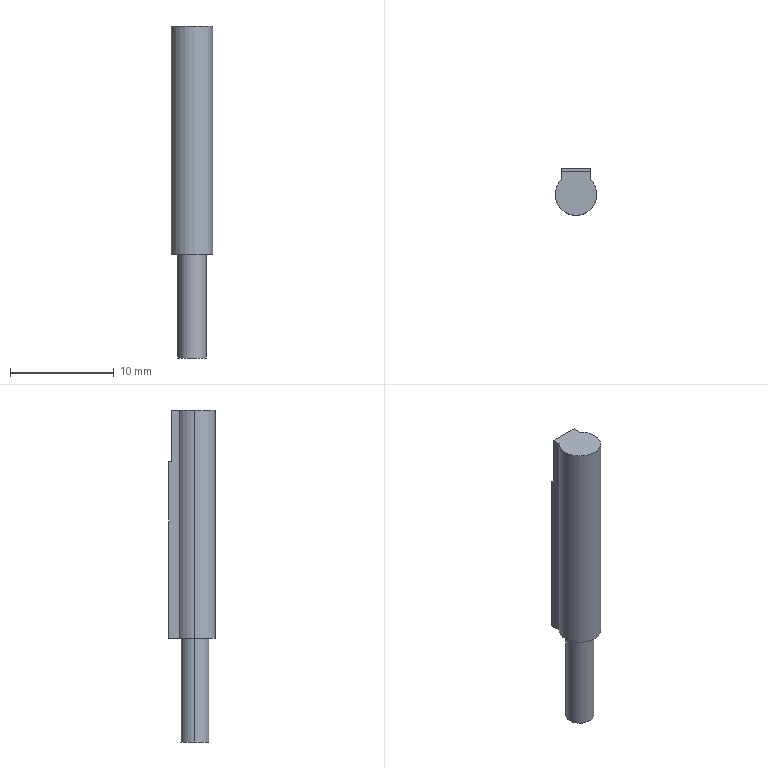Part | SolidWorks | features BaseBody 1 | 1 solid | 23 faces | box 4 x 4.5 x 32 mm | volume 371.041 mm3 | plane 13 | cylinder 10 | commonest cylinder face diameters 2.1 x3 4 x3 2.5 x2 2.7 x2
STEP:
#1=CARTESIAN_POINT('',(-1.35,0.,-22.));
#2=VERTEX_POINT('',#1);
#3=CARTESIAN_POINT('',(1.35,0.,-22.));
#4=VERTEX_POINT('',#3);
#5=CARTESIAN_POINT('',(0.,0.,-22.));
#6=DIRECTION('',(0.,0.,-1.));
#7=DIRECTION('',(1.,0.,0.));
#8=AXIS2_PLACEMENT_3D('',#5,#6,#7);
#9=CIRCLE('',#8,1.35);
#10=EDGE_CURVE('',#2,#4,#9,.T.);
#11=ORIENTED_EDGE('',*,*,#10,.T.);
#12=CARTESIAN_POINT('',(1.35,0.,-32.));
#13=VERTEX_POINT('',#12);
#14=CARTESIAN_POINT('',(1.35,0.,-32.));
#15=DIRECTION('',(0.,0.,-1.));
#16=VECTOR('',#15,1000.);
#17=LINE('',#14,#16);
#18=EDGE_CURVE('',#4,#13,#17,.T.);
#19=ORIENTED_EDGE('',*,*,#18,.T.);
#20=CARTESIAN_POINT('',(-1.35,0.,-32.));
#21=VERTEX_POINT('',#20);
#22=CARTESIAN_POINT('',(0.,0.,-32.));
#23=DIRECTION('',(0.,0.,-1.));
#24=DIRECTION('',(-1.,0.,0.));
#25=AXIS2_PLACEMENT_3D('',#22,#23,#24);
#26=CIRCLE('',#25,1.35);
#27=EDGE_CURVE('',#21,#13,#26,.T.);
#28=ORIENTED_EDGE('',*,*,#27,.F.);
#29=CARTESIAN_POINT('',(-1.35,0.,-32.));
#30=DIRECTION('',(0.,0.,-1.));
#31=VECTOR('',#30,1000.);
#32=LINE('',#29,#31);
#33=EDGE_CURVE('',#2,#21,#32,.T.);
#34=ORIENTED_EDGE('',*,*,#33,.F.);
#35=EDGE_LOOP('',(#11,#19,#28,#34));
#36=FACE_OUTER_BOUND('',#35,.T.);
#37=CARTESIAN_POINT('',(0.,0.,-32.));
#38=DIRECTION('',(0.,0.,-1.));
#39=DIRECTION('',(-1.,0.,0.));
#40=AXIS2_PLACEMENT_3D('',#37,#38,#39);
#41=CYLINDRICAL_SURFACE('',#40,1.35);
#42=ADVANCED_FACE('',(#36),#41,.T.);
#43=CARTESIAN_POINT('',(-1.4,1.428,-22.));
#44=VERTEX_POINT('',#43);
#45=CARTESIAN_POINT('',(-2.,0.,-22.));
#46=VERTEX_POINT('',#45);
#47=CARTESIAN_POINT('',(0.,0.,-22.));
#48=DIRECTION('',(0.,0.,1.));
#49=DIRECTION('',(-0.7,0.7141,0.));
#50=AXIS2_PLACEMENT_3D('',#47,#48,#49);
#51=CIRCLE('',#50,2.);
#52=EDGE_CURVE('',#44,#46,#51,.T.);
#53=ORIENTED_EDGE('',*,*,#52,.T.);
#54=CARTESIAN_POINT('',(-2.,0.,0.));
#55=VERTEX_POINT('',#54);
#56=CARTESIAN_POINT('',(-2.,0.,-22.));
#57=DIRECTION('',(0.,0.,1.));
#58=VECTOR('',#57,1000.);
#59=LINE('',#56,#58);
#60=EDGE_CURVE('',#46,#55,#59,.T.);
#61=ORIENTED_EDGE('',*,*,#60,.T.);
#62=CARTESIAN_POINT('',(-1.4,1.428,0.));
#63=VERTEX_POINT('',#62);
#64=CARTESIAN_POINT('',(0.,0.,0.));
#65=DIRECTION('',(0.,0.,1.));
#66=DIRECTION('',(-0.7,0.7141,0.));
#67=AXIS2_PLACEMENT_3D('',#64,#65,#66);
#68=CIRCLE('',#67,2.);
#69=EDGE_CURVE('',#63,#55,#68,.T.);
#70=ORIENTED_EDGE('',*,*,#69,.F.);
#71=CARTESIAN_POINT('',(-1.4,1.428,-22.));
#72=DIRECTION('',(0.,0.,1.));
#73=VECTOR('',#72,1000.);
#74=LINE('',#71,#73);
#75=EDGE_CURVE('',#44,#63,#74,.T.);
#76=ORIENTED_EDGE('',*,*,#75,.F.);
#77=EDGE_LOOP('',(#53,#61,#70,#76));
#78=FACE_OUTER_BOUND('',#77,.T.);
#79=CARTESIAN_POINT('',(0.,0.,-22.));
#80=DIRECTION('',(0.,0.,1.));
#81=DIRECTION('',(1.,0.,0.));
#82=AXIS2_PLACEMENT_3D('',#79,#80,#81);
#83=CYLINDRICAL_SURFACE('',#82,2.);
#84=ADVANCED_FACE('',(#78),#83,.T.);
#85=ORIENTED_EDGE('',*,*,#60,.F.);
#86=CARTESIAN_POINT('',(2.,0.,-22.));
#87=VERTEX_POINT('',#86);
#88=CARTESIAN_POINT('',(0.,0.,-22.));
#89=DIRECTION('',(0.,0.,1.));
#90=DIRECTION('',(-0.7,0.7141,0.));
#91=AXIS2_PLACEMENT_3D('',#88,#89,#90);
#92=CIRCLE('',#91,2.);
#93=EDGE_CURVE('',#46,#87,#92,.T.);
#94=ORIENTED_EDGE('',*,*,#93,.T.);
#95=CARTESIAN_POINT('',(2.,0.,0.));
#96=VERTEX_POINT('',#95);
#97=CARTESIAN_POINT('',(2.,0.,-22.));
#98=DIRECTION('',(0.,0.,1.));
#99=VECTOR('',#98,1000.);
#100=LINE('',#97,#99);
#101=EDGE_CURVE('',#87,#96,#100,.T.);
#102=ORIENTED_EDGE('',*,*,#101,.T.);
#103=CARTESIAN_POINT('',(0.,0.,0.));
#104=DIRECTION('',(0.,0.,1.));
#105=DIRECTION('',(-0.7,0.7141,0.));
#106=AXIS2_PLACEMENT_3D('',#103,#104,#105);
#107=CIRCLE('',#106,2.);
#108=EDGE_CURVE('',#55,#96,#107,.T.);
#109=ORIENTED_EDGE('',*,*,#108,.F.);
#110=EDGE_LOOP('',(#85,#94,#102,#109));
#111=FACE_OUTER_BOUND('',#110,.T.);
#112=CARTESIAN_POINT('',(0.,0.,-22.));
#113=DIRECTION('',(0.,0.,1.));
#114=DIRECTION('',(1.,0.,0.));
#115=AXIS2_PLACEMENT_3D('',#112,#113,#114);
#116=CYLINDRICAL_SURFACE('',#115,2.);
#117=ADVANCED_FACE('',(#111),#116,.T.);
#118=CARTESIAN_POINT('',(0.,2.1,-3.25));
#119=VERTEX_POINT('',#118);
#120=CARTESIAN_POINT('',(0.,2.1,-0.75));
#121=VERTEX_POINT('',#120);
#122=CARTESIAN_POINT('',(0.,2.1,-2.));
#123=DIRECTION('',(0.,1.,0.));
#124=DIRECTION('',(1.,0.,0.));
#125=AXIS2_PLACEMENT_3D('',#122,#123,#124);
#126=CIRCLE('',#125,1.25);
#127=EDGE_CURVE('',#119,#121,#126,.T.);
#128=ORIENTED_EDGE('',*,*,#127,.F.);
#129=CARTESIAN_POINT('',(0.,2.2,-3.25));
#130=VERTEX_POINT('',#129);
#131=CARTESIAN_POINT('',(0.,2.1,-3.25));
#132=DIRECTION('',(0.,1.,0.));
#133=VECTOR('',#132,1000.);
#134=LINE('',#131,#133);
#135=EDGE_CURVE('',#119,#130,#134,.T.);
#136=ORIENTED_EDGE('',*,*,#135,.T.);
#137=CARTESIAN_POINT('',(0.,2.2,-0.75));
#138=VERTEX_POINT('',#137);
#139=CARTESIAN_POINT('',(0.,2.2,-2.));
#140=DIRECTION('',(0.,1.,0.));
#141=DIRECTION('',(1.,0.,0.));
#142=AXIS2_PLACEMENT_3D('',#139,#140,#141);
#143=CIRCLE('',#142,1.25);
#144=EDGE_CURVE('',#130,#138,#143,.T.);
#145=ORIENTED_EDGE('',*,*,#144,.T.);
#146=CARTESIAN_POINT('',(0.,2.1,-0.75));
#147=DIRECTION('',(0.,1.,0.));
#148=VECTOR('',#147,1000.);
#149=LINE('',#146,#148);
#150=EDGE_CURVE('',#121,#138,#149,.T.);
#151=ORIENTED_EDGE('',*,*,#150,.F.);
#152=EDGE_LOOP('',(#128,#136,#145,#151));
#153=FACE_OUTER_BOUND('',#152,.T.);
#154=CARTESIAN_POINT('',(0.,2.1,-2.));
#155=DIRECTION('',(0.,1.,0.));
#156=DIRECTION('',(0.,0.,1.));
#157=AXIS2_PLACEMENT_3D('',#154,#155,#156);
#158=CYLINDRICAL_SURFACE('',#157,1.25);
#159=ADVANCED_FACE('',(#153),#158,.F.);
#160=CARTESIAN_POINT('',(-0.5443,2.1,-1.102));
#161=VERTEX_POINT('',#160);
#162=CARTESIAN_POINT('',(0.,2.1,-0.95));
#163=VERTEX_POINT('',#162);
#164=CARTESIAN_POINT('',(0.,2.1,-2.));
#165=DIRECTION('',(0.,1.,0.));
#166=DIRECTION('',(-0.5184,0.,0.8551));
#167=AXIS2_PLACEMENT_3D('',#164,#165,#166);
#168=CIRCLE('',#167,1.05);
#169=EDGE_CURVE('',#161,#163,#168,.T.);
#170=ORIENTED_EDGE('',*,*,#169,.T.);
#171=CARTESIAN_POINT('',(0.,2.2,-0.95));
#172=VERTEX_POINT('',#171);
#173=CARTESIAN_POINT('',(0.,2.1,-0.95));
#174=DIRECTION('',(0.,1.,0.));
#175=VECTOR('',#174,1000.);
#176=LINE('',#173,#175);
#177=EDGE_CURVE('',#163,#172,#176,.T.);
#178=ORIENTED_EDGE('',*,*,#177,.T.);
#179=CARTESIAN_POINT('',(-0.5443,2.2,-1.102));
#180=VERTEX_POINT('',#179);
#181=CARTESIAN_POINT('',(0.,2.2,-2.));
#182=DIRECTION('',(0.,1.,0.));
#183=DIRECTION('',(-0.5184,0.,0.8551));
#184=AXIS2_PLACEMENT_3D('',#181,#182,#183);
#185=CIRCLE('',#184,1.05);
#186=EDGE_CURVE('',#180,#172,#185,.T.);
#187=ORIENTED_EDGE('',*,*,#186,.F.);
#188=CARTESIAN_POINT('',(-0.5443,2.1,-1.102));
#189=DIRECTION('',(0.,1.,0.));
#190=VECTOR('',#189,1000.);
#191=LINE('',#188,#190);
#192=EDGE_CURVE('',#161,#180,#191,.T.);
#193=ORIENTED_EDGE('',*,*,#192,.F.);
#194=EDGE_LOOP('',(#170,#178,#187,#193));
#195=FACE_OUTER_BOUND('',#194,.T.);
#196=CARTESIAN_POINT('',(0.,2.1,-2.));
#197=DIRECTION('',(0.,1.,0.));
#198=DIRECTION('',(0.,0.,1.));
#199=AXIS2_PLACEMENT_3D('',#196,#197,#198);
#200=CYLINDRICAL_SURFACE('',#199,1.05);
#201=ADVANCED_FACE('',(#195),#200,.T.);
#202=CARTESIAN_POINT('',(-0.8979,2.1,-1.456));
#203=VERTEX_POINT('',#202);
#204=CARTESIAN_POINT('',(-0.8979,2.2,-1.456));
#205=VERTEX_POINT('',#204);
#206=CARTESIAN_POINT('',(-0.8979,2.1,-1.456));
#207=DIRECTION('',(0.,1.,0.));
#208=VECTOR('',#207,1000.);
#209=LINE('',#206,#208);
#210=EDGE_CURVE('',#203,#205,#209,.T.);
#211=ORIENTED_EDGE('',*,*,#210,.T.);
#212=CARTESIAN_POINT('',(0.5443,2.2,-2.898));
#213=VERTEX_POINT('',#212);
#214=CARTESIAN_POINT('',(0.,2.2,-2.));
#215=DIRECTION('',(0.,1.,0.));
#216=DIRECTION('',(0.5184,0.,-0.8551));
#217=AXIS2_PLACEMENT_3D('',#214,#215,#216);
#218=CIRCLE('',#217,1.05);
#219=EDGE_CURVE('',#213,#205,#218,.T.);
#220=ORIENTED_EDGE('',*,*,#219,.F.);
#221=CARTESIAN_POINT('',(0.5443,2.1,-2.898));
#222=VERTEX_POINT('',#221);
#223=CARTESIAN_POINT('',(0.5443,2.1,-2.898));
#224=DIRECTION('',(0.,1.,0.));
#225=VECTOR('',#224,1000.);
#226=LINE('',#223,#225);
#227=EDGE_CURVE('',#222,#213,#226,.T.);
#228=ORIENTED_EDGE('',*,*,#227,.F.);
#229=CARTESIAN_POINT('',(0.,2.1,-2.));
#230=DIRECTION('',(0.,1.,0.));
#231=DIRECTION('',(0.5184,0.,-0.8551));
#232=AXIS2_PLACEMENT_3D('',#229,#230,#231);
#233=CIRCLE('',#232,1.05);
#234=EDGE_CURVE('',#222,#203,#233,.T.);
#235=ORIENTED_EDGE('',*,*,#234,.T.);
#236=EDGE_LOOP('',(#211,#220,#228,#235));
#237=FACE_OUTER_BOUND('',#236,.T.);
#238=CARTESIAN_POINT('',(0.,2.1,-2.));
#239=DIRECTION('',(0.,1.,0.));
#240=DIRECTION('',(0.,0.,1.));
#241=AXIS2_PLACEMENT_3D('',#238,#239,#240);
#242=CYLINDRICAL_SURFACE('',#241,1.05);
#243=ADVANCED_FACE('',(#237),#242,.T.);
#244=CARTESIAN_POINT('',(0.5443,2.2,-2.898));
#245=DIRECTION('',(-0.7071,0.,0.7071));
#246=VECTOR('',#245,1000.);
#247=LINE('',#244,#246);
#248=EDGE_CURVE('',#213,#205,#247,.T.);
#249=ORIENTED_EDGE('',*,*,#248,.T.);
#250=ORIENTED_EDGE('',*,*,#210,.F.);
#251=CARTESIAN_POINT('',(0.5443,2.1,-2.898));
#252=DIRECTION('',(-0.7071,0.,0.7071));
#253=VECTOR('',#252,1000.);
#254=LINE('',#251,#253);
#255=EDGE_CURVE('',#222,#203,#254,.T.);
#256=ORIENTED_EDGE('',*,*,#255,.F.);
#257=ORIENTED_EDGE('',*,*,#227,.T.);
#258=EDGE_LOOP('',(#249,#250,#256,#257));
#259=FACE_OUTER_BOUND('',#258,.T.);
#260=CARTESIAN_POINT('',(0.5443,2.1,-2.898));
#261=DIRECTION('',(-0.7071,0.,-0.7071));
#262=DIRECTION('',(-0.7071,0.,0.7071));
#263=AXIS2_PLACEMENT_3D('',#260,#261,#262);
#264=PLANE('',#263);
#265=ADVANCED_FACE('',(#259),#264,.F.);
#266=ORIENTED_EDGE('',*,*,#219,.T.);
#267=ORIENTED_EDGE('',*,*,#248,.F.);
#268=EDGE_LOOP('',(#266,#267));
#269=FACE_OUTER_BOUND('',#268,.T.);
#270=CARTESIAN_POINT('',(-1.4,2.2,-5.));
#271=DIRECTION('',(0.,-1.,0.));
#272=DIRECTION('',(0.,0.,-1.));
#273=AXIS2_PLACEMENT_3D('',#270,#271,#272);
#274=PLANE('',#273);
#275=ADVANCED_FACE('',(#269),#274,.F.);
#276=ORIENTED_EDGE('',*,*,#169,.F.);
#277=CARTESIAN_POINT('',(0.8979,2.1,-2.544));
#278=VERTEX_POINT('',#277);
#279=CARTESIAN_POINT('',(-0.5443,2.1,-1.102));
#280=DIRECTION('',(0.7071,0.,-0.7071));
#281=VECTOR('',#280,1000.);
#282=LINE('',#279,#281);
#283=EDGE_CURVE('',#161,#278,#282,.T.);
#284=ORIENTED_EDGE('',*,*,#283,.T.);
#285=CARTESIAN_POINT('',(0.,2.1,-2.));
#286=DIRECTION('',(0.,1.,0.));
#287=DIRECTION('',(-0.5184,0.,0.8551));
#288=AXIS2_PLACEMENT_3D('',#285,#286,#287);
#289=CIRCLE('',#288,1.05);
#290=EDGE_CURVE('',#163,#278,#289,.T.);
#291=ORIENTED_EDGE('',*,*,#290,.F.);
#292=EDGE_LOOP('',(#276,#284,#291));
#293=FACE_BOUND('',#292,.T.);
#294=ORIENTED_EDGE('',*,*,#234,.F.);
#295=ORIENTED_EDGE('',*,*,#255,.T.);
#296=EDGE_LOOP('',(#294,#295));
#297=FACE_BOUND('',#296,.T.);
#298=CARTESIAN_POINT('',(0.,2.1,-2.));
#299=DIRECTION('',(0.,1.,0.));
#300=DIRECTION('',(1.,0.,0.));
#301=AXIS2_PLACEMENT_3D('',#298,#299,#300);
#302=CIRCLE('',#301,1.25);
#303=EDGE_CURVE('',#121,#119,#302,.T.);
#304=ORIENTED_EDGE('',*,*,#303,.T.);
#305=ORIENTED_EDGE('',*,*,#127,.T.);
#306=EDGE_LOOP('',(#304,#305));
#307=FACE_OUTER_BOUND('',#306,.T.);
#308=CARTESIAN_POINT('',(0.,2.1,-2.));
#309=DIRECTION('',(0.,1.,0.));
#310=DIRECTION('',(0.,0.,1.));
#311=AXIS2_PLACEMENT_3D('',#308,#309,#310);
#312=PLANE('',#311);
#313=ADVANCED_FACE('',(#293,#297,#307),#312,.T.);
#314=ORIENTED_EDGE('',*,*,#177,.F.);
#315=ORIENTED_EDGE('',*,*,#290,.T.);
#316=CARTESIAN_POINT('',(0.8979,2.2,-2.544));
#317=VERTEX_POINT('',#316);
#318=CARTESIAN_POINT('',(0.8979,2.1,-2.544));
#319=DIRECTION('',(0.,1.,0.));
#320=VECTOR('',#319,1000.);
#321=LINE('',#318,#320);
#322=EDGE_CURVE('',#278,#317,#321,.T.);
#323=ORIENTED_EDGE('',*,*,#322,.T.);
#324=CARTESIAN_POINT('',(0.,2.2,-2.));
#325=DIRECTION('',(0.,1.,0.));
#326=DIRECTION('',(-0.5184,0.,0.8551));
#327=AXIS2_PLACEMENT_3D('',#324,#325,#326);
#328=CIRCLE('',#327,1.05);
#329=EDGE_CURVE('',#172,#317,#328,.T.);
#330=ORIENTED_EDGE('',*,*,#329,.F.);
#331=EDGE_LOOP('',(#314,#315,#323,#330));
#332=FACE_OUTER_BOUND('',#331,.T.);
#333=CARTESIAN_POINT('',(0.,2.1,-2.));
#334=DIRECTION('',(0.,1.,0.));
#335=DIRECTION('',(0.,0.,1.));
#336=AXIS2_PLACEMENT_3D('',#333,#334,#335);
#337=CYLINDRICAL_SURFACE('',#336,1.05);
#338=ADVANCED_FACE('',(#332),#337,.T.);
#339=CARTESIAN_POINT('',(-0.5443,2.2,-1.102));
#340=DIRECTION('',(0.7071,0.,-0.7071));
#341=VECTOR('',#340,1000.);
#342=LINE('',#339,#341);
#343=EDGE_CURVE('',#180,#317,#342,.T.);
#344=ORIENTED_EDGE('',*,*,#343,.T.);
#345=ORIENTED_EDGE('',*,*,#322,.F.);
#346=ORIENTED_EDGE('',*,*,#283,.F.);
#347=ORIENTED_EDGE('',*,*,#192,.T.);
#348=EDGE_LOOP('',(#344,#345,#346,#347));
#349=FACE_OUTER_BOUND('',#348,.T.);
#350=CARTESIAN_POINT('',(-0.5443,2.1,-1.102));
#351=DIRECTION('',(0.7071,0.,0.7071));
#352=DIRECTION('',(0.7071,0.,-0.7071));
#353=AXIS2_PLACEMENT_3D('',#350,#351,#352);
#354=PLANE('',#353);
#355=ADVANCED_FACE('',(#349),#354,.F.);
#356=ORIENTED_EDGE('',*,*,#135,.F.);
#357=ORIENTED_EDGE('',*,*,#303,.F.);
#358=ORIENTED_EDGE('',*,*,#150,.T.);
#359=CARTESIAN_POINT('',(0.,2.2,-2.));
#360=DIRECTION('',(0.,1.,0.));
#361=DIRECTION('',(1.,0.,0.));
#362=AXIS2_PLACEMENT_3D('',#359,#360,#361);
#363=CIRCLE('',#362,1.25);
#364=EDGE_CURVE('',#138,#130,#363,.T.);
#365=ORIENTED_EDGE('',*,*,#364,.T.);
#366=EDGE_LOOP('',(#356,#357,#358,#365));
#367=FACE_OUTER_BOUND('',#366,.T.);
#368=CARTESIAN_POINT('',(0.,2.1,-2.));
#369=DIRECTION('',(0.,1.,0.));
#370=DIRECTION('',(0.,0.,1.));
#371=AXIS2_PLACEMENT_3D('',#368,#369,#370);
#372=CYLINDRICAL_SURFACE('',#371,1.25);
#373=ADVANCED_FACE('',(#367),#372,.F.);
#374=ORIENTED_EDGE('',*,*,#186,.T.);
#375=ORIENTED_EDGE('',*,*,#329,.T.);
#376=ORIENTED_EDGE('',*,*,#343,.F.);
#377=EDGE_LOOP('',(#374,#375,#376));
#378=FACE_OUTER_BOUND('',#377,.T.);
#379=CARTESIAN_POINT('',(-1.4,2.2,-5.));
#380=DIRECTION('',(0.,-1.,0.));
#381=DIRECTION('',(0.,0.,-1.));
#382=AXIS2_PLACEMENT_3D('',#379,#380,#381);
#383=PLANE('',#382);
#384=ADVANCED_FACE('',(#378),#383,.F.);
#385=ORIENTED_EDGE('',*,*,#364,.F.);
#386=ORIENTED_EDGE('',*,*,#144,.F.);
#387=EDGE_LOOP('',(#385,#386));
#388=FACE_BOUND('',#387,.T.);
#389=CARTESIAN_POINT('',(-1.4,2.2,0.));
#390=VERTEX_POINT('',#389);
#391=CARTESIAN_POINT('',(1.4,2.2,0.));
#392=VERTEX_POINT('',#391);
#393=CARTESIAN_POINT('',(-1.4,2.2,0.));
#394=DIRECTION('',(1.,0.,0.));
#395=VECTOR('',#394,1000.);
#396=LINE('',#393,#395);
#397=EDGE_CURVE('',#390,#392,#396,.T.);
#398=ORIENTED_EDGE('',*,*,#397,.T.);
#399=CARTESIAN_POINT('',(1.4,2.2,-5.));
#400=VERTEX_POINT('',#399);
#401=CARTESIAN_POINT('',(1.4,2.2,-5.));
#402=DIRECTION('',(0.,0.,1.));
#403=VECTOR('',#402,1000.);
#404=LINE('',#401,#403);
#405=EDGE_CURVE('',#400,#392,#404,.T.);
#406=ORIENTED_EDGE('',*,*,#405,.F.);
#407=CARTESIAN_POINT('',(-1.4,2.2,-5.));
#408=VERTEX_POINT('',#407);
#409=CARTESIAN_POINT('',(-1.4,2.2,-5.));
#410=DIRECTION('',(1.,0.,0.));
#411=VECTOR('',#410,1000.);
#412=LINE('',#409,#411);
#413=EDGE_CURVE('',#408,#400,#412,.T.);
#414=ORIENTED_EDGE('',*,*,#413,.F.);
#415=CARTESIAN_POINT('',(-1.4,2.2,-5.));
#416=DIRECTION('',(0.,0.,1.));
#417=VECTOR('',#416,1000.);
#418=LINE('',#415,#417);
#419=EDGE_CURVE('',#408,#390,#418,.T.);
#420=ORIENTED_EDGE('',*,*,#419,.T.);
#421=EDGE_LOOP('',(#398,#406,#414,#420));
#422=FACE_OUTER_BOUND('',#421,.T.);
#423=CARTESIAN_POINT('',(-1.4,2.2,-5.));
#424=DIRECTION('',(0.,-1.,0.));
#425=DIRECTION('',(0.,0.,-1.));
#426=AXIS2_PLACEMENT_3D('',#423,#424,#425);
#427=PLANE('',#426);
#428=ADVANCED_FACE('',(#388,#422),#427,.F.);
#429=ORIENTED_EDGE('',*,*,#397,.F.);
#430=CARTESIAN_POINT('',(-1.4,2.2,0.));
#431=DIRECTION('',(0.,-1.,0.));
#432=VECTOR('',#431,1000.);
#433=LINE('',#430,#432);
#434=EDGE_CURVE('',#390,#63,#433,.T.);
#435=ORIENTED_EDGE('',*,*,#434,.T.);
#436=ORIENTED_EDGE('',*,*,#69,.T.);
#437=ORIENTED_EDGE('',*,*,#108,.T.);
#438=CARTESIAN_POINT('',(1.4,1.428,0.));
#439=VERTEX_POINT('',#438);
#440=CARTESIAN_POINT('',(0.,0.,0.));
#441=DIRECTION('',(0.,0.,1.));
#442=DIRECTION('',(-0.7,0.7141,0.));
#443=AXIS2_PLACEMENT_3D('',#440,#441,#442);
#444=CIRCLE('',#443,2.);
#445=EDGE_CURVE('',#96,#439,#444,.T.);
#446=ORIENTED_EDGE('',*,*,#445,.T.);
#447=CARTESIAN_POINT('',(1.4,1.428,0.));
#448=DIRECTION('',(0.,1.,0.));
#449=VECTOR('',#448,1000.);
#450=LINE('',#447,#449);
#451=EDGE_CURVE('',#439,#392,#450,.T.);
#452=ORIENTED_EDGE('',*,*,#451,.T.);
#453=EDGE_LOOP('',(#429,#435,#436,#437,#446,#452));
#454=FACE_OUTER_BOUND('',#453,.T.);
#455=CARTESIAN_POINT('',(0.,0.,0.));
#456=DIRECTION('',(0.,0.,1.));
#457=DIRECTION('',(1.,0.,0.));
#458=AXIS2_PLACEMENT_3D('',#455,#456,#457);
#459=PLANE('',#458);
#460=ADVANCED_FACE('',(#454),#459,.T.);
#461=ORIENTED_EDGE('',*,*,#405,.T.);
#462=ORIENTED_EDGE('',*,*,#451,.F.);
#463=CARTESIAN_POINT('',(1.4,1.428,-22.));
#464=VERTEX_POINT('',#463);
#465=CARTESIAN_POINT('',(1.4,1.428,-22.));
#466=DIRECTION('',(0.,0.,1.));
#467=VECTOR('',#466,1000.);
#468=LINE('',#465,#467);
#469=EDGE_CURVE('',#464,#439,#468,.T.);
#470=ORIENTED_EDGE('',*,*,#469,.F.);
#471=CARTESIAN_POINT('',(1.4,2.5,-22.));
#472=VERTEX_POINT('',#471);
#473=CARTESIAN_POINT('',(1.4,1.428,-22.));
#474=DIRECTION('',(0.,1.,0.));
#475=VECTOR('',#474,1000.);
#476=LINE('',#473,#475);
#477=EDGE_CURVE('',#464,#472,#476,.T.);
#478=ORIENTED_EDGE('',*,*,#477,.T.);
#479=CARTESIAN_POINT('',(1.4,2.5,-5.));
#480=VERTEX_POINT('',#479);
#481=CARTESIAN_POINT('',(1.4,2.5,-22.));
#482=DIRECTION('',(0.,0.,1.));
#483=VECTOR('',#482,1000.);
#484=LINE('',#481,#483);
#485=EDGE_CURVE('',#472,#480,#484,.T.);
#486=ORIENTED_EDGE('',*,*,#485,.T.);
#487=CARTESIAN_POINT('',(1.4,2.2,-5.));
#488=DIRECTION('',(0.,1.,0.));
#489=VECTOR('',#488,1000.);
#490=LINE('',#487,#489);
#491=EDGE_CURVE('',#400,#480,#490,.T.);
#492=ORIENTED_EDGE('',*,*,#491,.F.);
#493=EDGE_LOOP('',(#461,#462,#470,#478,#486,#492));
#494=FACE_OUTER_BOUND('',#493,.T.);
#495=CARTESIAN_POINT('',(1.4,1.428,-22.));
#496=DIRECTION('',(1.,0.,0.));
#497=DIRECTION('',(0.,0.,-1.));
#498=AXIS2_PLACEMENT_3D('',#495,#496,#497);
#499=PLANE('',#498);
#500=ADVANCED_FACE('',(#494),#499,.T.);
#501=CARTESIAN_POINT('',(-1.4,2.5,-5.));
#502=VERTEX_POINT('',#501);
#503=CARTESIAN_POINT('',(-1.4,2.5,-5.));
#504=DIRECTION('',(0.,-1.,0.));
#505=VECTOR('',#504,1000.);
#506=LINE('',#503,#505);
#507=EDGE_CURVE('',#502,#408,#506,.T.);
#508=ORIENTED_EDGE('',*,*,#507,.T.);
#509=ORIENTED_EDGE('',*,*,#413,.T.);
#510=ORIENTED_EDGE('',*,*,#491,.T.);
#511=CARTESIAN_POINT('',(1.4,2.5,-5.));
#512=DIRECTION('',(-1.,0.,0.));
#513=VECTOR('',#512,1000.);
#514=LINE('',#511,#513);
#515=EDGE_CURVE('',#480,#502,#514,.T.);
#516=ORIENTED_EDGE('',*,*,#515,.T.);
#517=EDGE_LOOP('',(#508,#509,#510,#516));
#518=FACE_OUTER_BOUND('',#517,.T.);
#519=CARTESIAN_POINT('',(0.,0.,-5.));
#520=DIRECTION('',(0.,0.,1.));
#521=DIRECTION('',(1.,0.,0.));
#522=AXIS2_PLACEMENT_3D('',#519,#520,#521);
#523=PLANE('',#522);
#524=ADVANCED_FACE('',(#518),#523,.T.);
#525=ORIENTED_EDGE('',*,*,#419,.F.);
#526=ORIENTED_EDGE('',*,*,#507,.F.);
#527=CARTESIAN_POINT('',(-1.4,2.5,-22.));
#528=VERTEX_POINT('',#527);
#529=CARTESIAN_POINT('',(-1.4,2.5,-22.));
#530=DIRECTION('',(0.,0.,1.));
#531=VECTOR('',#530,1000.);
#532=LINE('',#529,#531);
#533=EDGE_CURVE('',#528,#502,#532,.T.);
#534=ORIENTED_EDGE('',*,*,#533,.F.);
#535=CARTESIAN_POINT('',(-1.4,2.5,-22.));
#536=DIRECTION('',(0.,-1.,0.));
#537=VECTOR('',#536,1000.);
#538=LINE('',#535,#537);
#539=EDGE_CURVE('',#528,#44,#538,.T.);
#540=ORIENTED_EDGE('',*,*,#539,.T.);
#541=ORIENTED_EDGE('',*,*,#75,.T.);
#542=ORIENTED_EDGE('',*,*,#434,.F.);
#543=EDGE_LOOP('',(#525,#526,#534,#540,#541,#542));
#544=FACE_OUTER_BOUND('',#543,.T.);
#545=CARTESIAN_POINT('',(-1.4,2.5,-22.));
#546=DIRECTION('',(-1.,0.,0.));
#547=DIRECTION('',(0.,0.,1.));
#548=AXIS2_PLACEMENT_3D('',#545,#546,#547);
#549=PLANE('',#548);
#550=ADVANCED_FACE('',(#544),#549,.T.);
#551=ORIENTED_EDGE('',*,*,#101,.F.);
#552=CARTESIAN_POINT('',(0.,0.,-22.));
#553=DIRECTION('',(0.,0.,1.));
#554=DIRECTION('',(-0.7,0.7141,0.));
#555=AXIS2_PLACEMENT_3D('',#552,#553,#554);
#556=CIRCLE('',#555,2.);
#557=EDGE_CURVE('',#87,#464,#556,.T.);
#558=ORIENTED_EDGE('',*,*,#557,.T.);
#559=ORIENTED_EDGE('',*,*,#469,.T.);
#560=ORIENTED_EDGE('',*,*,#445,.F.);
#561=EDGE_LOOP('',(#551,#558,#559,#560));
#562=FACE_OUTER_BOUND('',#561,.T.);
#563=CARTESIAN_POINT('',(0.,0.,-22.));
#564=DIRECTION('',(0.,0.,1.));
#565=DIRECTION('',(1.,0.,0.));
#566=AXIS2_PLACEMENT_3D('',#563,#564,#565);
#567=CYLINDRICAL_SURFACE('',#566,2.);
#568=ADVANCED_FACE('',(#562),#567,.T.);
#569=ORIENTED_EDGE('',*,*,#10,.F.);
#570=CARTESIAN_POINT('',(0.,0.,-22.));
#571=DIRECTION('',(0.,0.,-1.));
#572=DIRECTION('',(1.,0.,0.));
#573=AXIS2_PLACEMENT_3D('',#570,#571,#572);
#574=CIRCLE('',#573,1.35);
#575=EDGE_CURVE('',#4,#2,#574,.T.);
#576=ORIENTED_EDGE('',*,*,#575,.F.);
#577=EDGE_LOOP('',(#569,#576));
#578=FACE_BOUND('',#577,.T.);
#579=ORIENTED_EDGE('',*,*,#539,.F.);
#580=CARTESIAN_POINT('',(1.4,2.5,-22.));
#581=DIRECTION('',(-1.,0.,0.));
#582=VECTOR('',#581,1000.);
#583=LINE('',#580,#582);
#584=EDGE_CURVE('',#472,#528,#583,.T.);
#585=ORIENTED_EDGE('',*,*,#584,.F.);
#586=ORIENTED_EDGE('',*,*,#477,.F.);
#587=ORIENTED_EDGE('',*,*,#557,.F.);
#588=ORIENTED_EDGE('',*,*,#93,.F.);
#589=ORIENTED_EDGE('',*,*,#52,.F.);
#590=EDGE_LOOP('',(#579,#585,#586,#587,#588,#589));
#591=FACE_OUTER_BOUND('',#590,.T.);
#592=CARTESIAN_POINT('',(0.,0.,-22.));
#593=DIRECTION('',(0.,0.,1.));
#594=DIRECTION('',(1.,0.,0.));
#595=AXIS2_PLACEMENT_3D('',#592,#593,#594);
#596=PLANE('',#595);
#597=ADVANCED_FACE('',(#578,#591),#596,.F.);
#598=ORIENTED_EDGE('',*,*,#533,.T.);
#599=ORIENTED_EDGE('',*,*,#515,.F.);
#600=ORIENTED_EDGE('',*,*,#485,.F.);
#601=ORIENTED_EDGE('',*,*,#584,.T.);
#602=EDGE_LOOP('',(#598,#599,#600,#601));
#603=FACE_OUTER_BOUND('',#602,.T.);
#604=CARTESIAN_POINT('',(1.4,2.5,-22.));
#605=DIRECTION('',(0.,1.,0.));
#606=DIRECTION('',(0.,0.,1.));
#607=AXIS2_PLACEMENT_3D('',#604,#605,#606);
#608=PLANE('',#607);
#609=ADVANCED_FACE('',(#603),#608,.T.);
#610=ORIENTED_EDGE('',*,*,#18,.F.);
#611=ORIENTED_EDGE('',*,*,#575,.T.);
#612=ORIENTED_EDGE('',*,*,#33,.T.);
#613=CARTESIAN_POINT('',(0.,0.,-32.));
#614=DIRECTION('',(0.,0.,-1.));
#615=DIRECTION('',(-1.,0.,0.));
#616=AXIS2_PLACEMENT_3D('',#613,#614,#615);
#617=CIRCLE('',#616,1.35);
#618=EDGE_CURVE('',#13,#21,#617,.T.);
#619=ORIENTED_EDGE('',*,*,#618,.F.);
#620=EDGE_LOOP('',(#610,#611,#612,#619));
#621=FACE_OUTER_BOUND('',#620,.T.);
#622=CARTESIAN_POINT('',(0.,0.,-32.));
#623=DIRECTION('',(0.,0.,-1.));
#624=DIRECTION('',(-1.,0.,0.));
#625=AXIS2_PLACEMENT_3D('',#622,#623,#624);
#626=CYLINDRICAL_SURFACE('',#625,1.35);
#627=ADVANCED_FACE('',(#621),#626,.T.);
#628=ORIENTED_EDGE('',*,*,#27,.T.);
#629=ORIENTED_EDGE('',*,*,#618,.T.);
#630=EDGE_LOOP('',(#628,#629));
#631=FACE_OUTER_BOUND('',#630,.T.);
#632=CARTESIAN_POINT('',(-1.35,0.,-32.));
#633=DIRECTION('',(0.,0.,1.));
#634=DIRECTION('',(1.,0.,0.));
#635=AXIS2_PLACEMENT_3D('',#632,#633,#634);
#636=PLANE('',#635);
#637=ADVANCED_FACE('',(#631),#636,.F.);
#638=CLOSED_SHELL('',(#42,#84,#117,#159,#201,#243,#265,#275,#313,#338,#355,#373,#384,#428,#460,#500,#524,#550,#568,#597,#609,#627,#637));
#639=MANIFOLD_SOLID_BREP('',#638);
#640=CARTESIAN_POINT('',(0.,0.,0.));
#641=DIRECTION('',(0.,0.,1.));
#642=DIRECTION('',(1.,0.,0.));
#643=AXIS2_PLACEMENT_3D('',#640,#641,#642);
#644=(LENGTH_UNIT()NAMED_UNIT(*)SI_UNIT(.MILLI.,.METRE.));
#645=UNCERTAINTY_MEASURE_WITH_UNIT(LENGTH_MEASURE(0.00001),#644,'','');
#646=(NAMED_UNIT(*)PLANE_ANGLE_UNIT()SI_UNIT($,.RADIAN.));
#647=(NAMED_UNIT(*)SI_UNIT($,.STERADIAN.)SOLID_ANGLE_UNIT());
#648=(GEOMETRIC_REPRESENTATION_CONTEXT(3)GLOBAL_UNCERTAINTY_ASSIGNED_CONTEXT((#645))GLOBAL_UNIT_ASSIGNED_CONTEXT((#644,#646,#647))REPRESENTATION_CONTEXT('',''));
#649=ADVANCED_BREP_SHAPE_REPRESENTATION('',(#639,#643),#648);